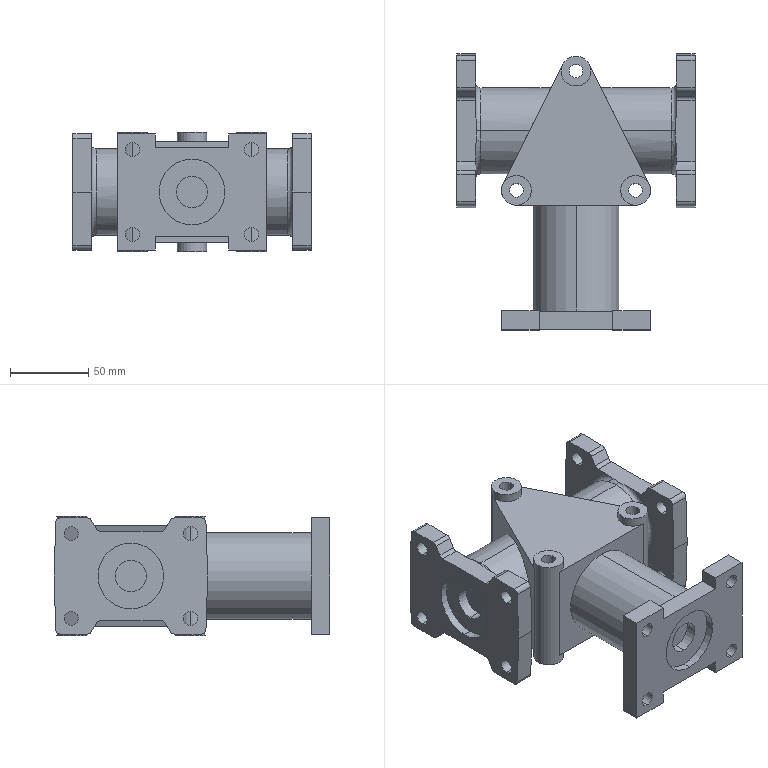Part | STEP file | 0244_Z_102_ARA610LR_1 | 1 solid | 148 faces | box 152 x 176 x 76 mm | volume 868653 mm3 | cylinder 79 | plane 65 | torus 4 | commonest cylinder face diameters 6 x24 9 x24 19 x7 8.8 x6 20 x6 42 x6